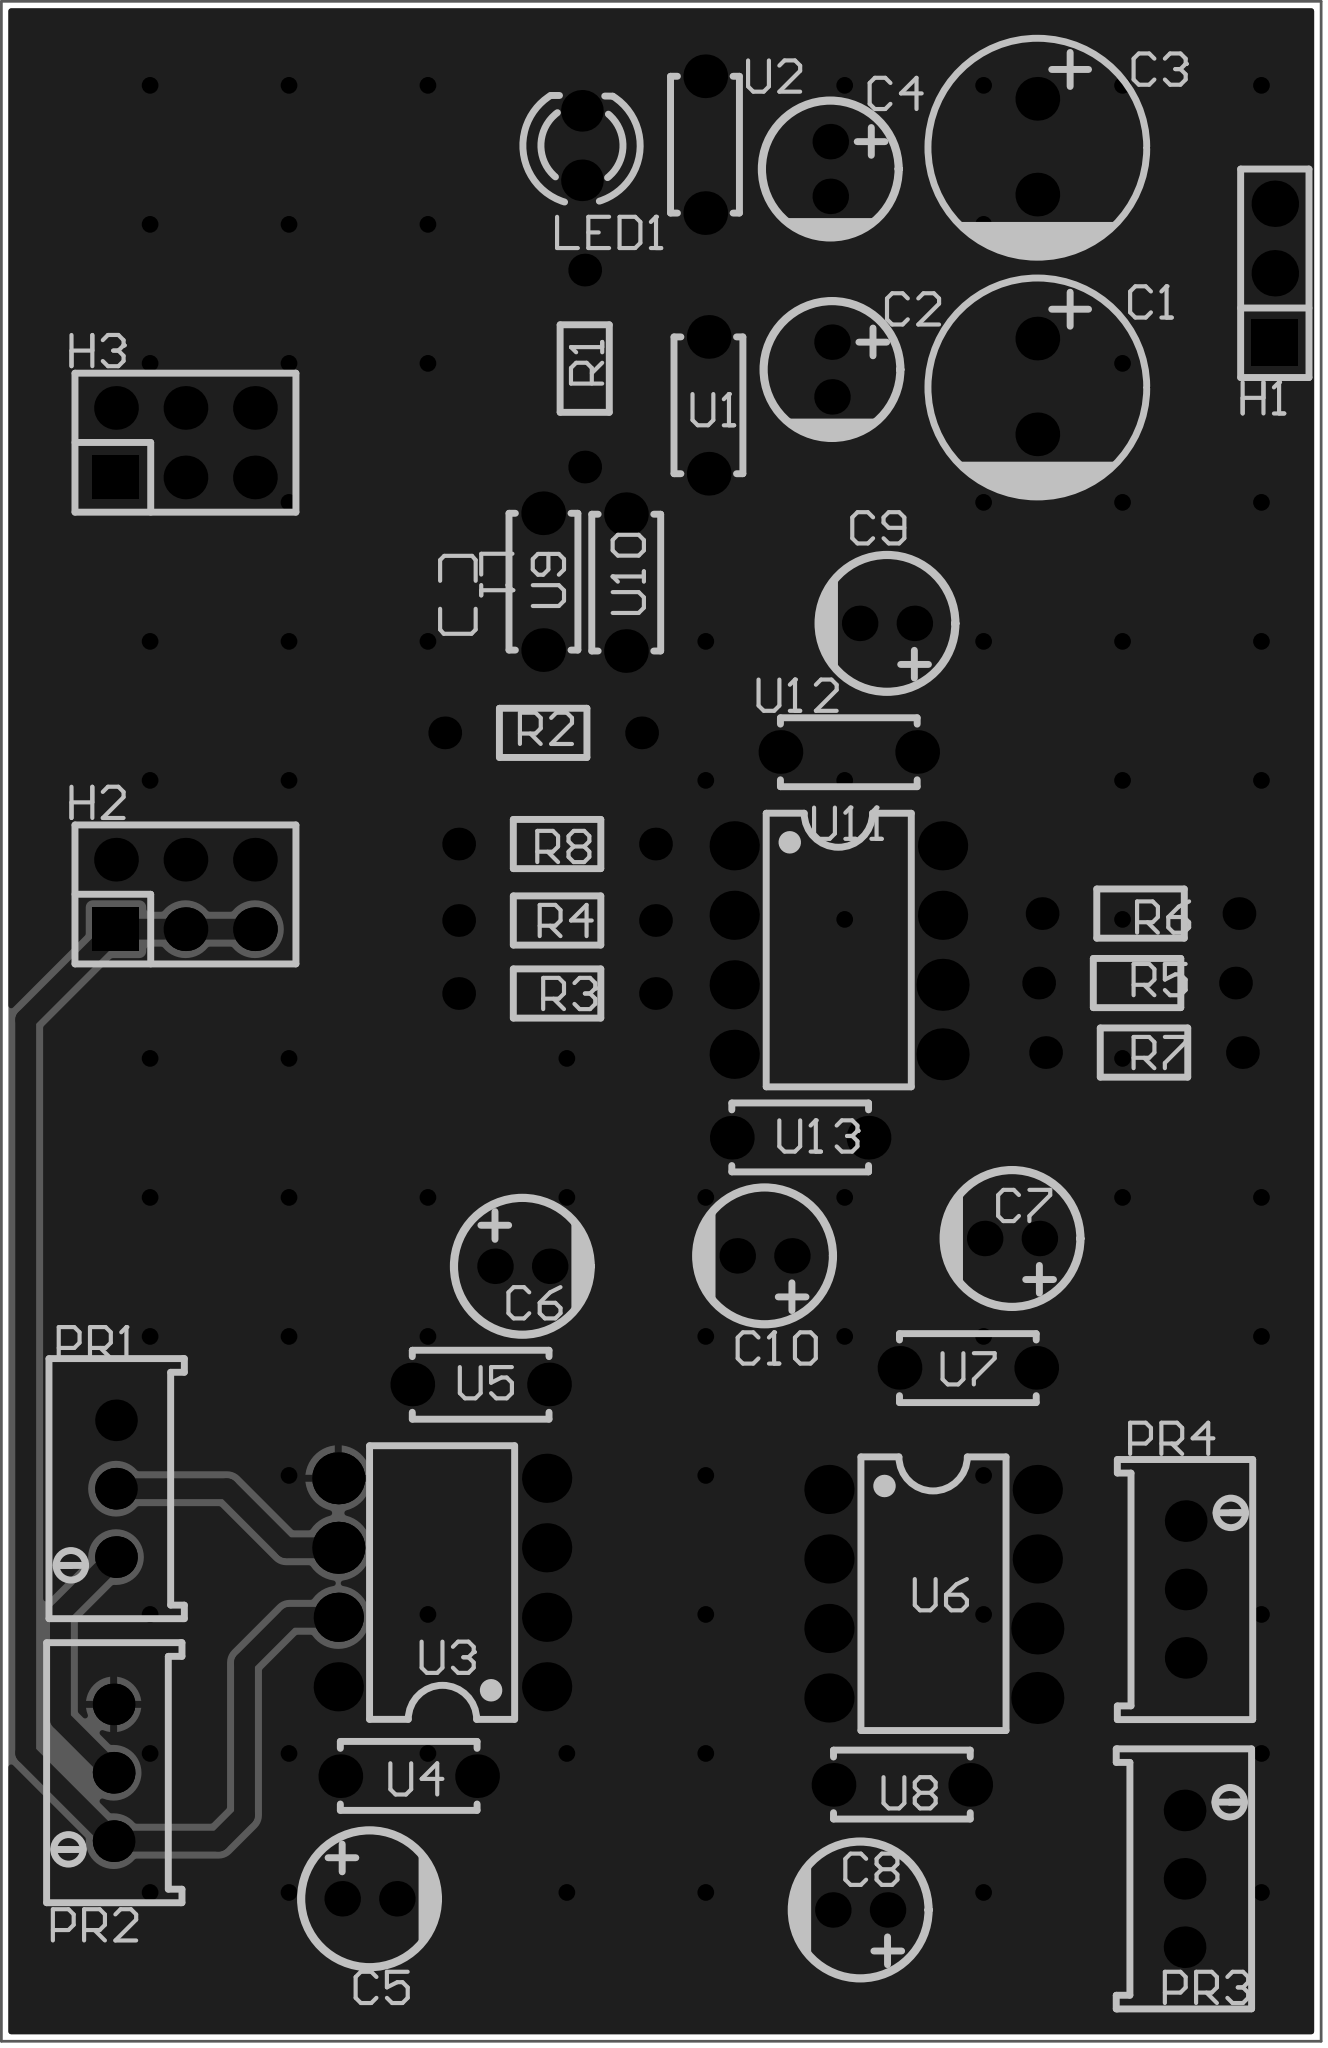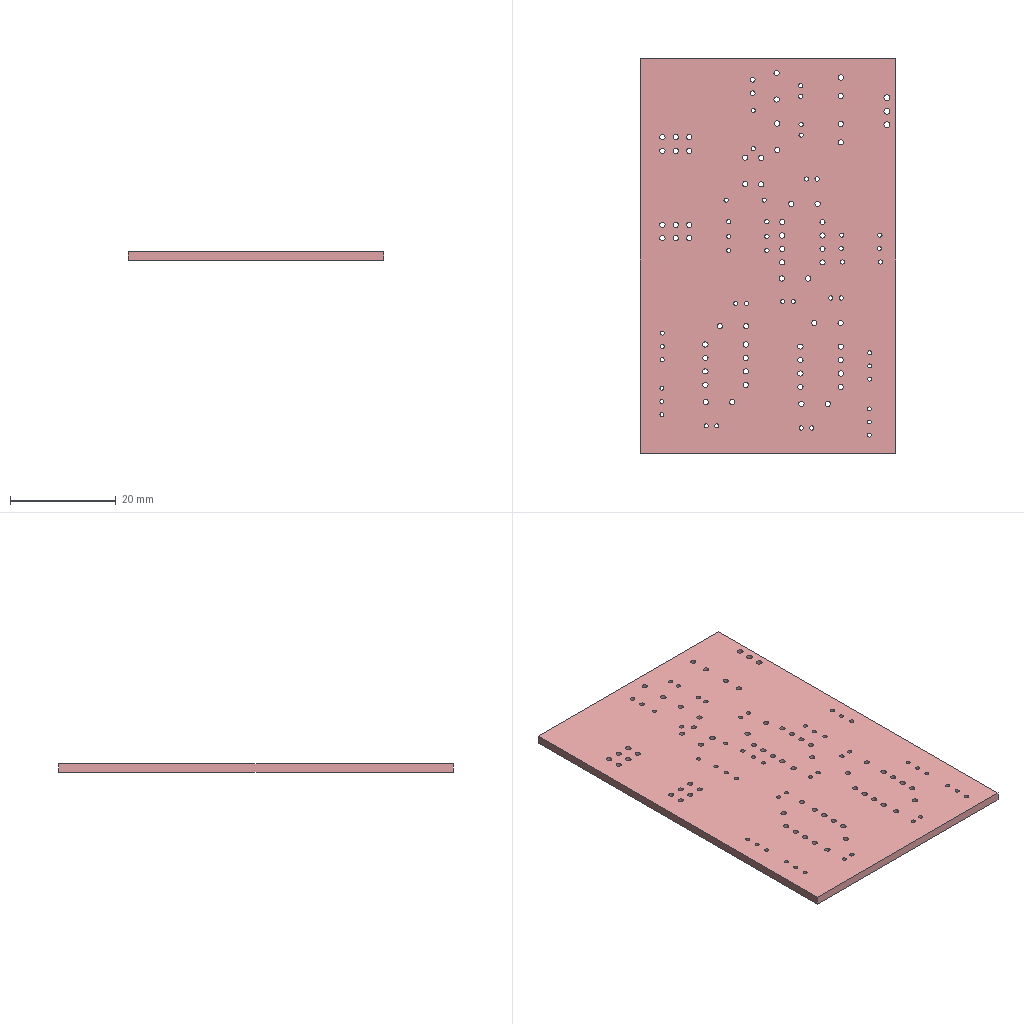Circuit board layout | Altium Designer | box 48.3 x 74.5 x 1.6 mm
Layer stack:
# Altium Designer layer stack of  (unit mm; dielectric type: 0 none, 1 core, 2 prepreg, 3 surface material)
index,name,kind,layer,copper_thickness_mm,dielectric_type,dielectric_thickness_mm,dielectric_material,dielectric_constant
0,Top Paste Mask Layer,other,,,,,,
1,Top Silkscreen Layer,other,,,,,,
2,Top Solder Mask Layer,dielectric,,,3,0.01,,3.3
3,Top Layer,copper,Top Layer,0.035,,,,
4,Dielectric1,dielectric,,,3,1.51,FR4,4.5
5,Bottom Layer,copper,Bottom Layer,0.035,,,,
6,Bottom Solder Mask Layer,dielectric,,,3,0.01,,3.3
7,Bottom Silkscreen Layer,other,,,,,,
8,Bottom Paste Mask Layer,other,,,,,,
# drill layer pairs: low layer,high layer
drill_pair,Top Layer,Bottom Layer
Part placement:
Designator,Comment,Layer,Footprint,Center-X(mm),Center-Y(mm),Rotation
C1,100uF,TopLayer,CAP-TH_BD8.0-P3.50-D0.6-FD_1,122.718,145.565,270
C2,10uF,TopLayer,CAP-TH_BD5.0-P2.00-D0.8-FD-10UF50VC110GL,115.209,146.184,270
C3,100uF,TopLayer,CAP-TH_BD8.0-P3.50-D0.6-FD_1,122.718,154.326,270
C4,10uF,TopLayer,CAP-TH_BD5.0-P2.00-D0.8-FD-10UF50VC110GL,115.147,153.511,270
C5,10uF,TopLayer,CAP-TH_BD5.0-P2.00-D0.8-FD-10UF50VC110GL,98.298,90.297,0
C6,10uF,TopLayer,CAP-TH_BD5.0-P2.00-D0.8-FD-10UF50VC110GL,103.886,113.411,0
C7,10uF,TopLayer,CAP-TH_BD5.0-P2.00-D0.8-FD-10UF50VC110GL,121.793,114.427,180
C8,10uF,TopLayer,CAP-TH_BD5.0-P2.00-D0.8-FD-10UF50VC110GL,116.24,89.888,180
C9,10uF,TopLayer,CAP-TH_BD5.0-P2.00-D0.8-FD-10UF50VC110GL,117.221,136.906,180
C10,10uF,TopLayer,CAP-TH_BD5.0-P2.00-D0.8-FD-10UF50VC110GL,112.744,113.792,180
H1,,TopLayer,HDR-TH_3P-P2.54-V-M,131.403,149.701,90
H2,,TopLayer,HDR-TH_6P-P2.54-V-F-R2-C3-S2.54,91.567,127,0
H3,,TopLayer,HDR-TH_6P-P2.54-V-F-R2-C3-S2.54,91.567,143.51,0
L1,20mH,TopLayer,L0603,101.529,137.95,270
LED1,,TopLayer,LED_TH-3mm,106.065,154.368,90
PR1,5kΩ,TopLayer,R_3296,89.027,105.283,90
PR2,200Ω,TopLayer,R_3296,88.941,94.902,90
PR3,5kΩ,TopLayer,R_3296,128.102,91.026,270
PR4,200Ω,TopLayer,R_3296,128.143,101.6,270
R1,20kΩ,TopLayer,Res_1/8W,106.166,146.219,90
R2,10kΩ,TopLayer,Res_1/8W,104.648,132.905,0
R3,10kΩ,TopLayer,Res_1/8W,105.156,123.38,0
R4,10kΩ,TopLayer,Res_1/8W,105.156,126.048,180
R5,10kΩ,TopLayer,Res_1/8W,126.365,123.762,180
R6,10kΩ,TopLayer,Res_1/8W,126.492,126.301,0
R7,10kΩ,TopLayer,Res_1/8W,126.619,121.222,180
R8,10kΩ,TopLayer,Res_1/8W,105.156,128.842,180
U1,100nF,TopLayer,CAP-TH_L5.0-W2.5-P5.00-D1.0,110.701,144.875,270
U2,100nF,TopLayer,CAP-TH_L5.0-W2.5-P5.00-D1.0,110.575,154.4,270
U3,NE5532AP,TopLayer,PDIP-8_L9.6-W6.4-P2.54-LS7.6-BL,100.965,101.854,90
U4,100nF,TopLayer,CAP-TH_L5.0-W2.5-P5.00-D1.0,99.731,94.777,180
U5,100nF,TopLayer,CAP-TH_L5.0-W2.5-P5.00-D1.0,102.362,109.093,0
U6,NE5532AP,TopLayer,PDIP-8_L9.6-W6.4-P2.54-LS7.6-BL,118.907,101.445,270
U7,100nF,TopLayer,CAP-TH_L5.0-W2.5-P5.00-D1.0,120.177,109.7,0
U8,100nF,TopLayer,CAP-TH_L5.0-W2.5-P5.00-D1.0,117.765,94.46,180
U9,100nF,TopLayer,CAP-TH_L5.0-W2.5-P5.00-D1.0,104.648,138.43,90
U10,100nF,TopLayer,CAP-TH_L5.0-W2.5-P5.00-D1.0,107.675,138.396,90
U11,NE5532AP,TopLayer,PDIP-8_L9.6-W6.4-P2.54-LS7.6-BL,115.443,124.968,270
U12,100nF,TopLayer,CAP-TH_L5.0-W2.5-P5.00-D1.0,115.824,132.207,0
U13,100nF,TopLayer,CAP-TH_L5.0-W2.5-P5.00-D1.0,114.046,118.11,180
Pad and via stacks:
# Altium Designer via and pad stacks of  (unit mm). Each distinct definition once, with the count of objects using it.
# via: kind,start_layer,end_layer,hole_mm,diameter_mm,mode(0 simple;1 top-mid-bottom;2 full stack),diameter_per_layer,count,example_net
# pad: kind,layer,hole_mm,hole_type(0 round;1 square;2 slot),plating,top_size,top_shape(1 round;2 rect;3 octagon;9 rounded rect),mid_size,bottom_size,mode,footprint,size_per_layer,count,example
pad,Multi-Layer,1,0,plated,1.6x1.6,1,1.6x1.6,1.6x1.6,0,CAP-TH_BD8.0-P3.50-D0.6-FD_1,,4,C1.2
pad,Multi-Layer,0.8,0,plated,1.3x1.3,1,1.3x1.3,1.3x1.3,0,CAP-TH_BD5.0-P2.00-D0.8-FD-10UF50VC110GL,,16,C2.2
pad,Multi-Layer,1.1,0,plated,1.7x1.7,2,1.7x1.7,1.7x1.7,0,HDR-TH_3P-P2.54-V-M,,1,H1.1
pad,Multi-Layer,1.1,0,plated,1.7x1.7,1,1.7x1.7,1.7x1.7,0,HDR-TH_3P-P2.54-V-M,,2,H1.2
pad,Multi-Layer,1,0,plated,1.7x1.6,2,1.7x1.6,1.7x1.6,0,HDR-TH_6P-P2.54-V-F-R2-C3-S2.54,,2,H2.1
pad,Multi-Layer,1,0,plated,1.6x1.6,1,1.6x1.6,1.6x1.6,0,HDR-TH_6P-P2.54-V-F-R2-C3-S2.54,,10,H2.2
pad,Multi-Layer,0.9144,0,plated,1.524x1.524,1,1.524x1.524,1.524x1.524,0,LED_TH-3mm,,2,LED1.1
pad,Multi-Layer,0.762,0,plated,1.524x1.524,1,1.524x1.524,1.524x1.524,0,R_3296,,12,PR1.2
pad,Multi-Layer,0.8001,0,plated,1.199x1.199,1,1.199x1.199,1.199x1.199,0,Res_1/8W,,16,R1.1
pad,Multi-Layer,1,0,plated,1.6x1.6,1,1.6x1.6,1.6x1.6,0,CAP-TH_L5.0-W2.5-P5.00-D1.0,,20,U1.1
pad,Multi-Layer,1,0,plated,1.8x1.8,1,1.8x1.8,1.8x1.8,0,PDIP-8_L9.6-W6.4-P2.54-LS7.6-BL,,18,U3.1
pad,Multi-Layer,1,0,plated,1.905x1.905,1,1.905x1.905,1.905x1.905,0,PDIP-8_L9.6-W6.4-P2.54-LS7.6-BL,,6,U3.5
pad,Top Layer,0,0,plated,0.8x0.864,2,0.8x0.864,0.8x0.864,0,L0603,,2,L1.1
via,Top Layer,Bottom Layer,0.3048,0.61,0,,73,GND
Copper pours:
name,layer,net,type(0 solid;1 hatched;2 none)
Top Layer-GND,Top Layer,GND,0
Bottom Layer-GND,Bottom Layer,GND,0
Design rules, without the lines most boards share:
# Altium Designer design rules of  (exported by Altium Designer, unit mm)
# columns: name | kind | enabled | priority | scope1 | scope2 | descriptor | typed fields (field=value)
creepage | 65 | enabled | 1 | All | All | Creepage Distance Constraint =(0mil) (All),(All) |